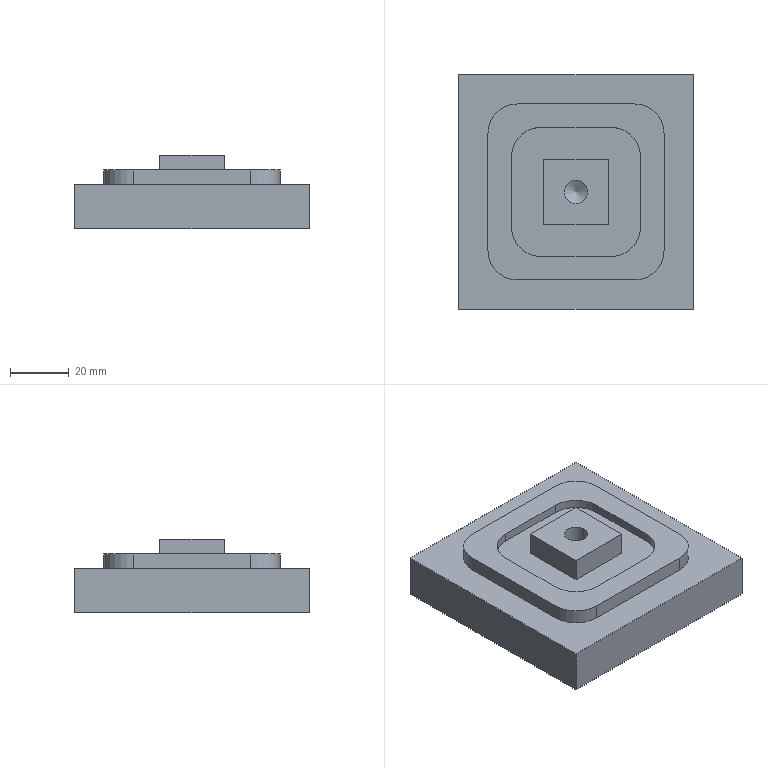CAM job | NX | 3-axis milling, drilling | part box 80 x 80 x 25 mm | stock box 80 x 80 x 25 mm
Tools:
number,name,description,diameter,corner_radius,flute_length,length,flutes
1,T1D12,Milling Tool-5 Parameters,12.0,0.0,50.0,75.0,2
2,T2D6,Milling Tool-5 Parameters,6.0,0.0,50.0,75.0,2
3,T3Z8,Drilling Tool,8.0,0.0,35.0,50.0,2
0,SPOTDRILLING_TOOL_Z10,Drilling Tool,10.0,0.0,35.0,50.0,2
Operations:
program,operation,operation_type,tool,method,geometry_group,spindle_rpm,surface_speed,feed_per_tooth,feed_cut,feed_plunge,cut_length_mm,path_length_mm,cut_time_min,machine_time_min
NC_PROGRAM,PLANAR_MILL,PlanarMilling,T1D12,MILL_ROUGH,WORKPIECE,2000.0,75.0,0.0625,1500.0,100.0,6806.329,6840.029,4.538,4.541
NC_PROGRAM,PLANAR_MILL_1,PlanarMilling,T1D12,MILL_ROUGH,WORKPIECE,1500.0,56.0,0.0833,1200.0,100.0,2734.524,2857.346,2.279,2.291
NC_PROGRAM,PLANAR_MILL_2,PlanarMilling,T2D6,MILL_ROUGH,WORKPIECE,2000.0,37.0,0.0625,1000.0,100.0,1257.74,1297.704,1.258,1.262
NC_PROGRAM,PLANAR_MILL_COPY,PlanarMilling,T1D12,MILL_FINISH,WORKPIECE,80.0,3.0,9.375,100.0,100.0,964.777,998.777,9.648,9.651
NC_PROGRAM,PLANAR_MILL_1_COPY,PlanarMilling,T1D12,MILL_FINISH,WORKPIECE,1500.0,56.0,0.0833,1200.0,100.0,529.562,557.562,0.4413,0.4441
NC_PROGRAM,PLANAR_MILL_2_COPY,PlanarMilling,T2D6,MILL_FINISH,WORKPIECE,100.0,1.0,5.0,200.0,100.0,833.253,883.153,4.166,4.171
NC_PROGRAM,SPOT_DRILLING,Operation,SPOTDRILLING_TOOL_Z10,DRILL_METHOD,WORKPIECE,0.0,0.0,0.0,200.0,0.0,10.0,20.0,0.0,0.001
NC_PROGRAM,DRILLING,Operation,T3Z8,DRILL_METHOD,WORKPIECE,100.0,2.0,0.75,85.0,0.0,10.0,20.0,0.0,0.001